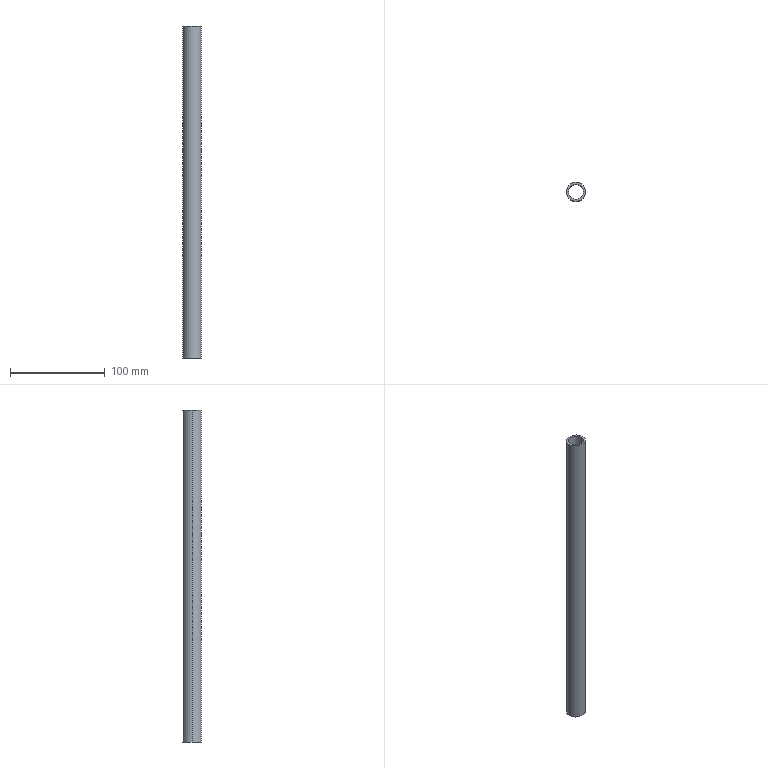Part | SolidWorks | features ExtruThin 1 | 1 solid | 6 faces | box 20 x 20 x 350 mm | volume 39584 mm3 | cylinder 4 | plane 2 | commonest cylinder face diameters 16 x2 20 x2
STEP:
#1=CARTESIAN_POINT('',(-8.,0.,350.));
#2=VERTEX_POINT('',#1);
#3=CARTESIAN_POINT('',(8.,0.,350.));
#4=VERTEX_POINT('',#3);
#5=CARTESIAN_POINT('',(0.,0.,350.));
#6=DIRECTION('',(0.,0.,1.));
#7=DIRECTION('',(1.,0.,0.));
#8=AXIS2_PLACEMENT_3D('',#5,#6,#7);
#9=CIRCLE('',#8,8.);
#10=EDGE_CURVE('',#2,#4,#9,.T.);
#11=ORIENTED_EDGE('',*,*,#10,.T.);
#12=CARTESIAN_POINT('',(8.,0.,0.));
#13=VERTEX_POINT('',#12);
#14=CARTESIAN_POINT('',(8.,0.,350.));
#15=DIRECTION('',(0.,0.,-1.));
#16=VECTOR('',#15,1000.);
#17=LINE('',#14,#16);
#18=EDGE_CURVE('',#4,#13,#17,.T.);
#19=ORIENTED_EDGE('',*,*,#18,.T.);
#20=CARTESIAN_POINT('',(-8.,0.,0.));
#21=VERTEX_POINT('',#20);
#22=CARTESIAN_POINT('',(0.,0.,0.));
#23=DIRECTION('',(0.,0.,1.));
#24=DIRECTION('',(1.,0.,0.));
#25=AXIS2_PLACEMENT_3D('',#22,#23,#24);
#26=CIRCLE('',#25,8.);
#27=EDGE_CURVE('',#21,#13,#26,.T.);
#28=ORIENTED_EDGE('',*,*,#27,.F.);
#29=CARTESIAN_POINT('',(-8.,0.,350.));
#30=DIRECTION('',(0.,0.,-1.));
#31=VECTOR('',#30,1000.);
#32=LINE('',#29,#31);
#33=EDGE_CURVE('',#2,#21,#32,.T.);
#34=ORIENTED_EDGE('',*,*,#33,.F.);
#35=EDGE_LOOP('',(#11,#19,#28,#34));
#36=FACE_OUTER_BOUND('',#35,.T.);
#37=CARTESIAN_POINT('',(0.,0.,350.));
#38=DIRECTION('',(0.,0.,-1.));
#39=DIRECTION('',(-1.,0.,0.));
#40=AXIS2_PLACEMENT_3D('',#37,#38,#39);
#41=CYLINDRICAL_SURFACE('',#40,8.);
#42=ADVANCED_FACE('',(#36),#41,.F.);
#43=CARTESIAN_POINT('',(10.,0.,350.));
#44=VERTEX_POINT('',#43);
#45=CARTESIAN_POINT('',(-10.,0.,350.));
#46=VERTEX_POINT('',#45);
#47=CARTESIAN_POINT('',(0.,0.,350.));
#48=DIRECTION('',(0.,0.,1.));
#49=DIRECTION('',(1.,0.,0.));
#50=AXIS2_PLACEMENT_3D('',#47,#48,#49);
#51=CIRCLE('',#50,10.);
#52=EDGE_CURVE('',#44,#46,#51,.T.);
#53=ORIENTED_EDGE('',*,*,#52,.F.);
#54=CARTESIAN_POINT('',(10.,0.,0.));
#55=VERTEX_POINT('',#54);
#56=CARTESIAN_POINT('',(10.,0.,350.));
#57=DIRECTION('',(0.,0.,-1.));
#58=VECTOR('',#57,1000.);
#59=LINE('',#56,#58);
#60=EDGE_CURVE('',#44,#55,#59,.T.);
#61=ORIENTED_EDGE('',*,*,#60,.T.);
#62=CARTESIAN_POINT('',(-10.,0.,0.));
#63=VERTEX_POINT('',#62);
#64=CARTESIAN_POINT('',(0.,0.,0.));
#65=DIRECTION('',(0.,0.,1.));
#66=DIRECTION('',(1.,0.,0.));
#67=AXIS2_PLACEMENT_3D('',#64,#65,#66);
#68=CIRCLE('',#67,10.);
#69=EDGE_CURVE('',#55,#63,#68,.T.);
#70=ORIENTED_EDGE('',*,*,#69,.T.);
#71=CARTESIAN_POINT('',(-10.,0.,350.));
#72=DIRECTION('',(0.,0.,-1.));
#73=VECTOR('',#72,1000.);
#74=LINE('',#71,#73);
#75=EDGE_CURVE('',#46,#63,#74,.T.);
#76=ORIENTED_EDGE('',*,*,#75,.F.);
#77=EDGE_LOOP('',(#53,#61,#70,#76));
#78=FACE_OUTER_BOUND('',#77,.T.);
#79=CARTESIAN_POINT('',(0.,0.,350.));
#80=DIRECTION('',(0.,0.,-1.));
#81=DIRECTION('',(-1.,0.,0.));
#82=AXIS2_PLACEMENT_3D('',#79,#80,#81);
#83=CYLINDRICAL_SURFACE('',#82,10.);
#84=ADVANCED_FACE('',(#78),#83,.T.);
#85=CARTESIAN_POINT('',(0.,0.,350.));
#86=DIRECTION('',(0.,0.,1.));
#87=DIRECTION('',(1.,0.,0.));
#88=AXIS2_PLACEMENT_3D('',#85,#86,#87);
#89=CIRCLE('',#88,10.);
#90=EDGE_CURVE('',#46,#44,#89,.T.);
#91=ORIENTED_EDGE('',*,*,#90,.T.);
#92=ORIENTED_EDGE('',*,*,#52,.T.);
#93=EDGE_LOOP('',(#91,#92));
#94=FACE_OUTER_BOUND('',#93,.T.);
#95=ORIENTED_EDGE('',*,*,#10,.F.);
#96=CARTESIAN_POINT('',(0.,0.,350.));
#97=DIRECTION('',(0.,0.,1.));
#98=DIRECTION('',(1.,0.,0.));
#99=AXIS2_PLACEMENT_3D('',#96,#97,#98);
#100=CIRCLE('',#99,8.);
#101=EDGE_CURVE('',#4,#2,#100,.T.);
#102=ORIENTED_EDGE('',*,*,#101,.F.);
#103=EDGE_LOOP('',(#95,#102));
#104=FACE_BOUND('',#103,.T.);
#105=CARTESIAN_POINT('',(0.,0.,350.));
#106=DIRECTION('',(0.,0.,1.));
#107=DIRECTION('',(1.,0.,0.));
#108=AXIS2_PLACEMENT_3D('',#105,#106,#107);
#109=PLANE('',#108);
#110=ADVANCED_FACE('',(#94,#104),#109,.T.);
#111=CARTESIAN_POINT('',(0.,0.,0.));
#112=DIRECTION('',(0.,0.,1.));
#113=DIRECTION('',(1.,0.,0.));
#114=AXIS2_PLACEMENT_3D('',#111,#112,#113);
#115=CIRCLE('',#114,10.);
#116=EDGE_CURVE('',#63,#55,#115,.T.);
#117=ORIENTED_EDGE('',*,*,#116,.F.);
#118=ORIENTED_EDGE('',*,*,#69,.F.);
#119=EDGE_LOOP('',(#117,#118));
#120=FACE_OUTER_BOUND('',#119,.T.);
#121=ORIENTED_EDGE('',*,*,#27,.T.);
#122=CARTESIAN_POINT('',(0.,0.,0.));
#123=DIRECTION('',(0.,0.,1.));
#124=DIRECTION('',(1.,0.,0.));
#125=AXIS2_PLACEMENT_3D('',#122,#123,#124);
#126=CIRCLE('',#125,8.);
#127=EDGE_CURVE('',#13,#21,#126,.T.);
#128=ORIENTED_EDGE('',*,*,#127,.T.);
#129=EDGE_LOOP('',(#121,#128));
#130=FACE_BOUND('',#129,.T.);
#131=CARTESIAN_POINT('',(0.,0.,0.));
#132=DIRECTION('',(0.,0.,1.));
#133=DIRECTION('',(1.,0.,0.));
#134=AXIS2_PLACEMENT_3D('',#131,#132,#133);
#135=PLANE('',#134);
#136=ADVANCED_FACE('',(#120,#130),#135,.F.);
#137=ORIENTED_EDGE('',*,*,#60,.F.);
#138=ORIENTED_EDGE('',*,*,#90,.F.);
#139=ORIENTED_EDGE('',*,*,#75,.T.);
#140=ORIENTED_EDGE('',*,*,#116,.T.);
#141=EDGE_LOOP('',(#137,#138,#139,#140));
#142=FACE_OUTER_BOUND('',#141,.T.);
#143=CARTESIAN_POINT('',(0.,0.,350.));
#144=DIRECTION('',(0.,0.,-1.));
#145=DIRECTION('',(-1.,0.,0.));
#146=AXIS2_PLACEMENT_3D('',#143,#144,#145);
#147=CYLINDRICAL_SURFACE('',#146,10.);
#148=ADVANCED_FACE('',(#142),#147,.T.);
#149=ORIENTED_EDGE('',*,*,#18,.F.);
#150=ORIENTED_EDGE('',*,*,#101,.T.);
#151=ORIENTED_EDGE('',*,*,#33,.T.);
#152=ORIENTED_EDGE('',*,*,#127,.F.);
#153=EDGE_LOOP('',(#149,#150,#151,#152));
#154=FACE_OUTER_BOUND('',#153,.T.);
#155=CARTESIAN_POINT('',(0.,0.,350.));
#156=DIRECTION('',(0.,0.,-1.));
#157=DIRECTION('',(-1.,0.,0.));
#158=AXIS2_PLACEMENT_3D('',#155,#156,#157);
#159=CYLINDRICAL_SURFACE('',#158,8.);
#160=ADVANCED_FACE('',(#154),#159,.F.);
#161=CLOSED_SHELL('',(#42,#84,#110,#136,#148,#160));
#162=MANIFOLD_SOLID_BREP('',#161);
#163=CARTESIAN_POINT('',(0.,0.,0.));
#164=DIRECTION('',(0.,0.,1.));
#165=DIRECTION('',(1.,0.,0.));
#166=AXIS2_PLACEMENT_3D('',#163,#164,#165);
#167=(LENGTH_UNIT()NAMED_UNIT(*)SI_UNIT(.MILLI.,.METRE.));
#168=UNCERTAINTY_MEASURE_WITH_UNIT(LENGTH_MEASURE(0.00001),#167,'','');
#169=(NAMED_UNIT(*)PLANE_ANGLE_UNIT()SI_UNIT($,.RADIAN.));
#170=(NAMED_UNIT(*)SI_UNIT($,.STERADIAN.)SOLID_ANGLE_UNIT());
#171=(GEOMETRIC_REPRESENTATION_CONTEXT(3)GLOBAL_UNCERTAINTY_ASSIGNED_CONTEXT((#168))GLOBAL_UNIT_ASSIGNED_CONTEXT((#167,#169,#170))REPRESENTATION_CONTEXT('',''));
#172=ADVANCED_BREP_SHAPE_REPRESENTATION('',(#162,#166),#171);